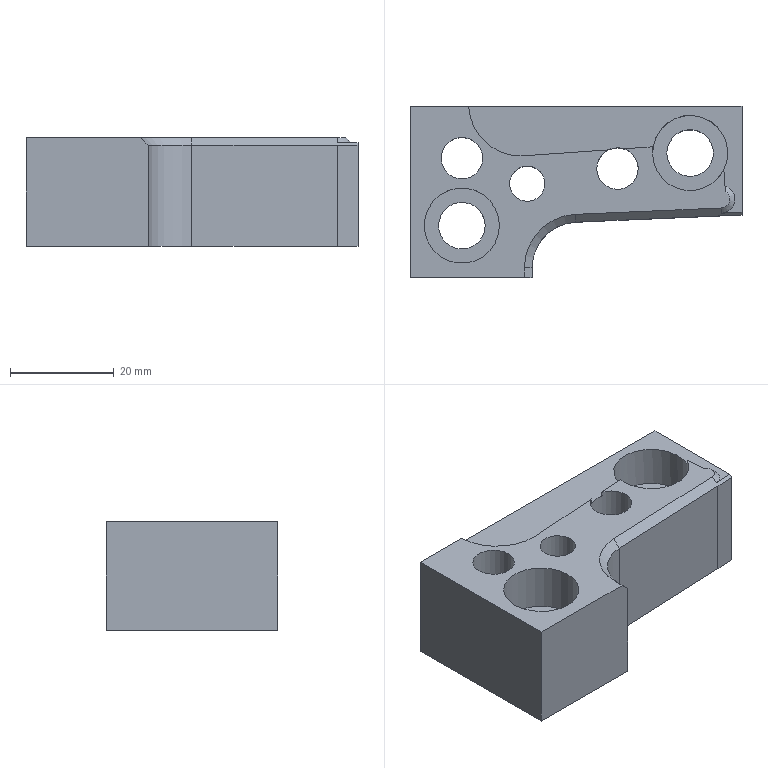Part | NX | features 23 2 | 1 solid | 28 faces | box 64 x 33 x 21 mm | volume 27332 mm3 | plane 17 | cylinder 9 | cone 2 | commonest cylinder face diameters 8.001 x2 9 x2 14.5 x2 6.8 x1 17.6 x1 19.999 x1
STEP:
#1=CARTESIAN_POINT('',(1071.25,364.,-2.5));
#2=VERTEX_POINT('',#1);
#3=CARTESIAN_POINT('',(1064.,364.,-2.5));
#4=DIRECTION('',(0.,0.,-1.));
#5=DIRECTION('',(1.,0.,0.));
#6=AXIS2_PLACEMENT_3D('',#3,#4,#5);
#7=CIRCLE('',#6,7.25);
#8=EDGE_CURVE('',#2,#2,#7,.T.);
#9=ORIENTED_EDGE('',*,*,#8,.T.);
#10=EDGE_LOOP('',(#9));
#11=FACE_BOUND('',#10,.T.);
#12=CARTESIAN_POINT('',(1068.001,377.,-2.5));
#13=VERTEX_POINT('',#12);
#14=CARTESIAN_POINT('',(1064.,377.,-2.5));
#15=DIRECTION('',(0.,0.,-1.));
#16=DIRECTION('',(1.,0.,0.));
#17=AXIS2_PLACEMENT_3D('',#14,#15,#16);
#18=CIRCLE('',#17,4.);
#19=EDGE_CURVE('',#13,#13,#18,.T.);
#20=ORIENTED_EDGE('',*,*,#19,.T.);
#21=EDGE_LOOP('',(#20));
#22=FACE_BOUND('',#21,.T.);
#23=CARTESIAN_POINT('',(1075.608,377.443,-2.5));
#24=VERTEX_POINT('',#23);
#25=CARTESIAN_POINT('',(1092.264,378.604,-2.5));
#26=VERTEX_POINT('',#25);
#27=CARTESIAN_POINT('',(1521.796,408.549,-2.5));
#28=DIRECTION('',(0.9976,0.06955,0.));
#29=VECTOR('',#28,1000.);
#30=LINE('',#27,#29);
#31=EDGE_CURVE('',#24,#26,#30,.T.);
#32=ORIENTED_EDGE('',*,*,#31,.F.);
#33=CARTESIAN_POINT('',(1065.29,387.,-2.5));
#34=VERTEX_POINT('',#33);
#35=CARTESIAN_POINT('',(1075.28,387.437,-2.5));
#36=DIRECTION('',(0.,0.,1.));
#37=DIRECTION('',(1.,0.,0.));
#38=AXIS2_PLACEMENT_3D('',#35,#36,#37);
#39=CIRCLE('',#38,10.);
#40=EDGE_CURVE('',#34,#24,#39,.T.);
#41=ORIENTED_EDGE('',*,*,#40,.F.);
#42=CARTESIAN_POINT('',(1054.,387.,-2.5));
#43=VERTEX_POINT('',#42);
#44=CARTESIAN_POINT('',(1136.,387.,-2.5));
#45=DIRECTION('',(-1.,0.,0.));
#46=VECTOR('',#45,1000.);
#47=LINE('',#44,#46);
#48=EDGE_CURVE('',#34,#43,#47,.T.);
#49=ORIENTED_EDGE('',*,*,#48,.T.);
#50=CARTESIAN_POINT('',(1054.,354.,-2.5));
#51=VERTEX_POINT('',#50);
#52=CARTESIAN_POINT('',(1054.,328.5,-2.5));
#53=DIRECTION('',(0.,-1.,0.));
#54=VECTOR('',#53,1000.);
#55=LINE('',#52,#54);
#56=EDGE_CURVE('',#43,#51,#55,.T.);
#57=ORIENTED_EDGE('',*,*,#56,.T.);
#58=CARTESIAN_POINT('',(1076.041,354.,-2.5));
#59=VERTEX_POINT('',#58);
#60=CARTESIAN_POINT('',(1166.5,354.,-2.5));
#61=DIRECTION('',(-1.,0.,0.));
#62=VECTOR('',#61,1000.);
#63=LINE('',#60,#62);
#64=EDGE_CURVE('',#59,#51,#63,.T.);
#65=ORIENTED_EDGE('',*,*,#64,.F.);
#66=CARTESIAN_POINT('',(1076.041,355.884,-2.5));
#67=VERTEX_POINT('',#66);
#68=CARTESIAN_POINT('',(1076.041,-425.,-2.5));
#69=DIRECTION('',(0.,1.,0.));
#70=VECTOR('',#69,1000.);
#71=LINE('',#68,#70);
#72=EDGE_CURVE('',#59,#67,#71,.T.);
#73=ORIENTED_EDGE('',*,*,#72,.T.);
#74=CARTESIAN_POINT('',(1085.893,366.175,-2.5));
#75=VERTEX_POINT('',#74);
#76=CARTESIAN_POINT('',(1086.341,355.884,-2.5));
#77=DIRECTION('',(0.,0.,1.));
#78=DIRECTION('',(1.,0.,0.));
#79=AXIS2_PLACEMENT_3D('',#76,#77,#78);
#80=CIRCLE('',#79,10.3);
#81=EDGE_CURVE('',#75,#67,#80,.T.);
#82=ORIENTED_EDGE('',*,*,#81,.F.);
#83=CARTESIAN_POINT('',(1113.99,367.4,-2.5));
#84=VERTEX_POINT('',#83);
#85=CARTESIAN_POINT('',(1544.537,386.173,-2.5));
#86=DIRECTION('',(0.9991,0.04356,0.));
#87=VECTOR('',#86,1000.);
#88=LINE('',#85,#87);
#89=EDGE_CURVE('',#75,#84,#88,.T.);
#90=ORIENTED_EDGE('',*,*,#89,.T.);
#91=CARTESIAN_POINT('',(1114.808,370.545,-2.5));
#92=VERTEX_POINT('',#91);
#93=CARTESIAN_POINT('',(1113.916,369.098,-2.5));
#94=DIRECTION('',(0.,0.,1.));
#95=DIRECTION('',(1.,0.,0.));
#96=AXIS2_PLACEMENT_3D('',#93,#94,#95);
#97=CIRCLE('',#96,1.7);
#98=EDGE_CURVE('',#84,#92,#97,.T.);
#99=ORIENTED_EDGE('',*,*,#98,.T.);
#100=CARTESIAN_POINT('',(1114.485,374.758,-2.5));
#101=VERTEX_POINT('',#100);
#102=CARTESIAN_POINT('',(1178.225,-455.826,-2.5));
#103=DIRECTION('',(0.07652,-0.9971,0.));
#104=VECTOR('',#103,1000.);
#105=LINE('',#102,#104);
#106=EDGE_CURVE('',#101,#92,#105,.T.);
#107=ORIENTED_EDGE('',*,*,#106,.F.);
#108=CARTESIAN_POINT('',(1100.85,379.203,-2.5));
#109=VERTEX_POINT('',#108);
#110=CARTESIAN_POINT('',(1108.,378.,-2.5));
#111=DIRECTION('',(0.,0.,-1.));
#112=DIRECTION('',(1.,0.,0.));
#113=AXIS2_PLACEMENT_3D('',#110,#111,#112);
#114=CIRCLE('',#113,7.25);
#115=EDGE_CURVE('',#101,#109,#114,.T.);
#116=ORIENTED_EDGE('',*,*,#115,.T.);
#117=CARTESIAN_POINT('',(1095.22,378.81,-2.5));
#118=VERTEX_POINT('',#117);
#119=CARTESIAN_POINT('',(1521.796,408.549,-2.5));
#120=DIRECTION('',(0.9976,0.06955,0.));
#121=VECTOR('',#120,1000.);
#122=LINE('',#119,#121);
#123=EDGE_CURVE('',#118,#109,#122,.T.);
#124=ORIENTED_EDGE('',*,*,#123,.F.);
#125=CARTESIAN_POINT('',(1094.,375.,-2.5));
#126=DIRECTION('',(0.,0.,-1.));
#127=DIRECTION('',(1.,0.,0.));
#128=AXIS2_PLACEMENT_3D('',#125,#126,#127);
#129=CIRCLE('',#128,4.);
#130=EDGE_CURVE('',#118,#26,#129,.T.);
#131=ORIENTED_EDGE('',*,*,#130,.T.);
#132=EDGE_LOOP('',(#32,#41,#49,#57,#65,#73,#82,#90,#99,#107,#116,#124,#131));
#133=FACE_BOUND('',#132,.T.);
#134=CARTESIAN_POINT('',(1079.999,372.088,-2.5));
#135=VERTEX_POINT('',#134);
#136=CARTESIAN_POINT('',(1076.599,372.088,-2.5));
#137=DIRECTION('',(0.,0.,1.));
#138=DIRECTION('',(1.,0.,0.));
#139=AXIS2_PLACEMENT_3D('',#136,#137,#138);
#140=CIRCLE('',#139,3.4);
#141=EDGE_CURVE('',#135,#135,#140,.T.);
#142=ORIENTED_EDGE('',*,*,#141,.F.);
#143=EDGE_LOOP('',(#142));
#144=FACE_BOUND('',#143,.T.);
#145=CARTESIAN_POINT('',(1166.5,279.5,-2.5));
#146=DIRECTION('',(0.,0.,1.));
#147=DIRECTION('',(-1.,0.,0.));
#148=AXIS2_PLACEMENT_3D('',#145,#146,#147);
#149=PLANE('',#148);
#150=ADVANCED_FACE('',(#11,#22,#133,#144),#149,.T.);
#151=ORIENTED_EDGE('',*,*,#123,.T.);
#152=CARTESIAN_POINT('',(1100.85,379.203,-3.5));
#153=VERTEX_POINT('',#152);
#154=CARTESIAN_POINT('',(1100.85,379.203,-3.5));
#155=DIRECTION('',(0.,0.,1.));
#156=VECTOR('',#155,1000.);
#157=LINE('',#154,#156);
#158=EDGE_CURVE('',#153,#109,#157,.T.);
#159=ORIENTED_EDGE('',*,*,#158,.F.);
#160=CARTESIAN_POINT('',(1095.22,378.81,-3.5));
#161=VERTEX_POINT('',#160);
#162=CARTESIAN_POINT('',(1580.768,412.66,-3.5));
#163=DIRECTION('',(0.9976,0.06955,0.));
#164=VECTOR('',#163,1000.);
#165=LINE('',#162,#164);
#166=EDGE_CURVE('',#161,#153,#165,.T.);
#167=ORIENTED_EDGE('',*,*,#166,.F.);
#168=CARTESIAN_POINT('',(1095.22,378.81,-0.5));
#169=DIRECTION('',(0.,0.,1.));
#170=VECTOR('',#169,1000.);
#171=LINE('',#168,#170);
#172=EDGE_CURVE('',#161,#118,#171,.T.);
#173=ORIENTED_EDGE('',*,*,#172,.T.);
#174=EDGE_LOOP('',(#151,#159,#167,#173));
#175=FACE_BOUND('',#174,.T.);
#176=CARTESIAN_POINT('',(1521.796,408.549,0.));
#177=DIRECTION('',(0.06955,-0.9976,0.));
#178=DIRECTION('',(0.9976,0.06955,0.));
#179=AXIS2_PLACEMENT_3D('',#176,#177,#178);
#180=PLANE('',#179);
#181=ADVANCED_FACE('',(#175),#180,.F.);
#182=CARTESIAN_POINT('',(1114.034,366.401,-3.5));
#183=VERTEX_POINT('',#182);
#184=CARTESIAN_POINT('',(1114.034,366.401,-3.5));
#185=DIRECTION('',(-0.0308,0.7064,0.7071));
#186=VECTOR('',#185,1000.);
#187=LINE('',#184,#186);
#188=EDGE_CURVE('',#183,#84,#187,.T.);
#189=ORIENTED_EDGE('',*,*,#188,.F.);
#190=CARTESIAN_POINT('',(1114.721,371.675,-3.5));
#191=VERTEX_POINT('',#190);
#192=CARTESIAN_POINT('',(1113.916,369.098,-3.5));
#193=DIRECTION('',(0.,0.,-1.));
#194=DIRECTION('',(-1.,0.,0.));
#195=AXIS2_PLACEMENT_3D('',#192,#193,#194);
#196=CIRCLE('',#195,2.7);
#197=EDGE_CURVE('',#191,#183,#196,.T.);
#198=ORIENTED_EDGE('',*,*,#197,.F.);
#199=CARTESIAN_POINT('',(1114.808,370.545,-2.5));
#200=CARTESIAN_POINT('',(1114.778,370.936,-2.817));
#201=CARTESIAN_POINT('',(1114.75,371.307,-3.157));
#202=CARTESIAN_POINT('',(1114.721,371.675,-3.5));
#203=B_SPLINE_CURVE_WITH_KNOTS('',3,(#199,#200,#201,#202),.UNSPECIFIED.,.F.,.F.,(4,4),(0.,0.001511),.UNSPECIFIED.);
#204=EDGE_CURVE('',#92,#191,#203,.T.);
#205=ORIENTED_EDGE('',*,*,#204,.F.);
#206=ORIENTED_EDGE('',*,*,#98,.F.);
#207=EDGE_LOOP('',(#189,#198,#205,#206));
#208=FACE_BOUND('',#207,.T.);
#209=CARTESIAN_POINT('',(1113.916,369.098,-3.5));
#210=DIRECTION('',(0.,0.,-1.));
#211=DIRECTION('',(-1.,0.,0.));
#212=AXIS2_PLACEMENT_3D('',#209,#210,#211);
#213=CONICAL_SURFACE('',#212,2.7,0.7854);
#214=ADVANCED_FACE('',(#208),#213,.T.);
#215=CARTESIAN_POINT('',(1065.29,387.,-3.5));
#216=VERTEX_POINT('',#215);
#217=CARTESIAN_POINT('',(1075.608,377.443,-3.5));
#218=VERTEX_POINT('',#217);
#219=CARTESIAN_POINT('',(1075.28,387.437,-3.5));
#220=DIRECTION('',(0.,0.,1.));
#221=DIRECTION('',(-1.,0.,0.));
#222=AXIS2_PLACEMENT_3D('',#219,#220,#221);
#223=CIRCLE('',#222,10.);
#224=EDGE_CURVE('',#216,#218,#223,.T.);
#225=ORIENTED_EDGE('',*,*,#224,.F.);
#226=CARTESIAN_POINT('',(1065.29,387.,0.));
#227=DIRECTION('',(0.,0.,-1.));
#228=VECTOR('',#227,1000.);
#229=LINE('',#226,#228);
#230=EDGE_CURVE('',#34,#216,#229,.T.);
#231=ORIENTED_EDGE('',*,*,#230,.F.);
#232=ORIENTED_EDGE('',*,*,#40,.T.);
#233=CARTESIAN_POINT('',(1075.608,377.443,-3.5));
#234=DIRECTION('',(0.,0.,-1.));
#235=VECTOR('',#234,1000.);
#236=LINE('',#233,#235);
#237=EDGE_CURVE('',#24,#218,#236,.T.);
#238=ORIENTED_EDGE('',*,*,#237,.T.);
#239=EDGE_LOOP('',(#225,#231,#232,#238));
#240=FACE_BOUND('',#239,.T.);
#241=CARTESIAN_POINT('',(1075.28,387.437,0.));
#242=DIRECTION('',(0.,0.,-1.));
#243=DIRECTION('',(-1.,0.,0.));
#244=AXIS2_PLACEMENT_3D('',#241,#242,#243);
#245=CYLINDRICAL_SURFACE('',#244,10.);
#246=ADVANCED_FACE('',(#240),#245,.F.);
#247=CARTESIAN_POINT('',(1092.264,378.604,-3.5));
#248=VERTEX_POINT('',#247);
#249=CARTESIAN_POINT('',(1092.264,378.604,-0.5));
#250=DIRECTION('',(0.,0.,-1.));
#251=VECTOR('',#250,1000.);
#252=LINE('',#249,#251);
#253=EDGE_CURVE('',#26,#248,#252,.T.);
#254=ORIENTED_EDGE('',*,*,#253,.T.);
#255=CARTESIAN_POINT('',(1580.768,412.66,-3.5));
#256=DIRECTION('',(0.9976,0.06955,0.));
#257=VECTOR('',#256,1000.);
#258=LINE('',#255,#257);
#259=EDGE_CURVE('',#218,#248,#258,.T.);
#260=ORIENTED_EDGE('',*,*,#259,.F.);
#261=ORIENTED_EDGE('',*,*,#237,.F.);
#262=ORIENTED_EDGE('',*,*,#31,.T.);
#263=EDGE_LOOP('',(#254,#260,#261,#262));
#264=FACE_BOUND('',#263,.T.);
#265=CARTESIAN_POINT('',(1521.796,408.549,0.));
#266=DIRECTION('',(0.06955,-0.9976,0.));
#267=DIRECTION('',(0.9976,0.06955,0.));
#268=AXIS2_PLACEMENT_3D('',#265,#266,#267);
#269=PLANE('',#268);
#270=ADVANCED_FACE('',(#264),#269,.F.);
#271=ORIENTED_EDGE('',*,*,#106,.T.);
#272=ORIENTED_EDGE('',*,*,#204,.T.);
#273=CARTESIAN_POINT('',(1114.485,374.758,-3.5));
#274=VERTEX_POINT('',#273);
#275=CARTESIAN_POINT('',(1113.377,389.198,-3.5));
#276=DIRECTION('',(0.07652,-0.9971,0.));
#277=VECTOR('',#276,1000.);
#278=LINE('',#275,#277);
#279=EDGE_CURVE('',#274,#191,#278,.T.);
#280=ORIENTED_EDGE('',*,*,#279,.F.);
#281=CARTESIAN_POINT('',(1114.485,374.758,-2.5));
#282=DIRECTION('',(0.,0.,-1.));
#283=VECTOR('',#282,1000.);
#284=LINE('',#281,#283);
#285=EDGE_CURVE('',#101,#274,#284,.T.);
#286=ORIENTED_EDGE('',*,*,#285,.F.);
#287=EDGE_LOOP('',(#271,#272,#280,#286));
#288=FACE_BOUND('',#287,.T.);
#289=CARTESIAN_POINT('',(1178.225,-455.826,0.));
#290=DIRECTION('',(-0.9971,-0.07652,0.));
#291=DIRECTION('',(0.07652,-0.9971,0.));
#292=AXIS2_PLACEMENT_3D('',#289,#290,#291);
#293=PLANE('',#292);
#294=ADVANCED_FACE('',(#288),#293,.F.);
#295=CARTESIAN_POINT('',(1118.,387.,-3.5));
#296=VERTEX_POINT('',#295);
#297=CARTESIAN_POINT('',(1118.,366.574,-3.5));
#298=VERTEX_POINT('',#297);
#299=CARTESIAN_POINT('',(1118.,332.,-3.5));
#300=DIRECTION('',(0.,-1.,0.));
#301=VECTOR('',#300,1000.);
#302=LINE('',#299,#301);
#303=EDGE_CURVE('',#296,#298,#302,.T.);
#304=ORIENTED_EDGE('',*,*,#303,.T.);
#305=CARTESIAN_POINT('',(1118.,366.073,-4.));
#306=VERTEX_POINT('',#305);
#307=CARTESIAN_POINT('',(1118.,351.02,-19.038));
#308=DIRECTION('',(0.,0.7074,0.7068));
#309=VECTOR('',#308,1000.);
#310=LINE('',#307,#309);
#311=EDGE_CURVE('',#306,#298,#310,.T.);
#312=ORIENTED_EDGE('',*,*,#311,.F.);
#313=CARTESIAN_POINT('',(1118.,366.073,-23.5));
#314=VERTEX_POINT('',#313);
#315=CARTESIAN_POINT('',(1118.,366.073,0.));
#316=DIRECTION('',(0.,0.,-1.));
#317=VECTOR('',#316,1000.);
#318=LINE('',#315,#317);
#319=EDGE_CURVE('',#306,#314,#318,.T.);
#320=ORIENTED_EDGE('',*,*,#319,.T.);
#321=CARTESIAN_POINT('',(1118.,387.,-23.5));
#322=VERTEX_POINT('',#321);
#323=CARTESIAN_POINT('',(1118.,328.5,-23.5));
#324=DIRECTION('',(0.,-1.,0.));
#325=VECTOR('',#324,1000.);
#326=LINE('',#323,#325);
#327=EDGE_CURVE('',#322,#314,#326,.T.);
#328=ORIENTED_EDGE('',*,*,#327,.F.);
#329=CARTESIAN_POINT('',(1118.,387.,-33.5));
#330=DIRECTION('',(0.,0.,1.));
#331=VECTOR('',#330,1000.);
#332=LINE('',#329,#331);
#333=EDGE_CURVE('',#322,#296,#332,.T.);
#334=ORIENTED_EDGE('',*,*,#333,.T.);
#335=EDGE_LOOP('',(#304,#312,#320,#328,#334));
#336=FACE_BOUND('',#335,.T.);
#337=CARTESIAN_POINT('',(1118.,332.,0.));
#338=DIRECTION('',(1.,0.,0.));
#339=DIRECTION('',(0.,0.,1.));
#340=AXIS2_PLACEMENT_3D('',#337,#338,#339);
#341=PLANE('',#340);
#342=ADVANCED_FACE('',(#336),#341,.T.);
#343=CARTESIAN_POINT('',(1073.199,372.088,-23.5));
#344=VERTEX_POINT('',#343);
#345=CARTESIAN_POINT('',(1076.599,372.088,-23.5));
#346=DIRECTION('',(0.,0.,1.));
#347=DIRECTION('',(-1.,0.,0.));
#348=AXIS2_PLACEMENT_3D('',#345,#346,#347);
#349=CIRCLE('',#348,3.4);
#350=EDGE_CURVE('',#344,#344,#349,.T.);
#351=ORIENTED_EDGE('',*,*,#350,.T.);
#352=EDGE_LOOP('',(#351));
#353=FACE_BOUND('',#352,.T.);
#354=CARTESIAN_POINT('',(1090.,375.,-23.5));
#355=VERTEX_POINT('',#354);
#356=CARTESIAN_POINT('',(1094.,375.,-23.5));
#357=DIRECTION('',(0.,0.,1.));
#358=DIRECTION('',(-1.,0.,0.));
#359=AXIS2_PLACEMENT_3D('',#356,#357,#358);
#360=CIRCLE('',#359,4.);
#361=EDGE_CURVE('',#355,#355,#360,.T.);
#362=ORIENTED_EDGE('',*,*,#361,.T.);
#363=EDGE_LOOP('',(#362));
#364=FACE_BOUND('',#363,.T.);
#365=CARTESIAN_POINT('',(1059.999,377.,-23.5));
#366=VERTEX_POINT('',#365);
#367=CARTESIAN_POINT('',(1064.,377.,-23.5));
#368=DIRECTION('',(0.,0.,1.));
#369=DIRECTION('',(-1.,0.,0.));
#370=AXIS2_PLACEMENT_3D('',#367,#368,#369);
#371=CIRCLE('',#370,4.);
#372=EDGE_CURVE('',#366,#366,#371,.T.);
#373=ORIENTED_EDGE('',*,*,#372,.T.);
#374=EDGE_LOOP('',(#373));
#375=FACE_BOUND('',#374,.T.);
#376=CARTESIAN_POINT('',(1059.5,364.,-23.5));
#377=VERTEX_POINT('',#376);
#378=CARTESIAN_POINT('',(1064.,364.,-23.5));
#379=DIRECTION('',(0.,0.,1.));
#380=DIRECTION('',(-1.,0.,0.));
#381=AXIS2_PLACEMENT_3D('',#378,#379,#380);
#382=CIRCLE('',#381,4.5);
#383=EDGE_CURVE('',#377,#377,#382,.T.);
#384=ORIENTED_EDGE('',*,*,#383,.T.);
#385=EDGE_LOOP('',(#384));
#386=FACE_BOUND('',#385,.T.);
#387=CARTESIAN_POINT('',(1103.5,378.,-23.5));
#388=VERTEX_POINT('',#387);
#389=CARTESIAN_POINT('',(1108.,378.,-23.5));
#390=DIRECTION('',(0.,0.,1.));
#391=DIRECTION('',(-1.,0.,0.));
#392=AXIS2_PLACEMENT_3D('',#389,#390,#391);
#393=CIRCLE('',#392,4.5);
#394=EDGE_CURVE('',#388,#388,#393,.T.);
#395=ORIENTED_EDGE('',*,*,#394,.T.);
#396=EDGE_LOOP('',(#395));
#397=FACE_BOUND('',#396,.T.);
#398=CARTESIAN_POINT('',(1054.,354.,-23.5));
#399=VERTEX_POINT('',#398);
#400=CARTESIAN_POINT('',(1077.541,354.,-23.5));
#401=VERTEX_POINT('',#400);
#402=CARTESIAN_POINT('',(1136.,354.,-23.5));
#403=DIRECTION('',(1.,0.,0.));
#404=VECTOR('',#403,1000.);
#405=LINE('',#402,#404);
#406=EDGE_CURVE('',#399,#401,#405,.T.);
#407=ORIENTED_EDGE('',*,*,#406,.F.);
#408=CARTESIAN_POINT('',(1054.,387.,-23.5));
#409=VERTEX_POINT('',#408);
#410=CARTESIAN_POINT('',(1054.,328.5,-23.5));
#411=DIRECTION('',(0.,1.,0.));
#412=VECTOR('',#411,1000.);
#413=LINE('',#410,#412);
#414=EDGE_CURVE('',#399,#409,#413,.T.);
#415=ORIENTED_EDGE('',*,*,#414,.T.);
#416=CARTESIAN_POINT('',(1136.,387.,-23.5));
#417=DIRECTION('',(1.,0.,0.));
#418=VECTOR('',#417,1000.);
#419=LINE('',#416,#418);
#420=EDGE_CURVE('',#409,#322,#419,.T.);
#421=ORIENTED_EDGE('',*,*,#420,.T.);
#422=ORIENTED_EDGE('',*,*,#327,.T.);
#423=CARTESIAN_POINT('',(1114.056,365.901,-23.5));
#424=VERTEX_POINT('',#423);
#425=CARTESIAN_POINT('',(1134.331,366.785,-23.5));
#426=DIRECTION('',(0.9991,0.04356,0.));
#427=VECTOR('',#426,1000.);
#428=LINE('',#425,#427);
#429=EDGE_CURVE('',#424,#314,#428,.T.);
#430=ORIENTED_EDGE('',*,*,#429,.F.);
#431=CARTESIAN_POINT('',(1085.958,364.676,-23.5));
#432=VERTEX_POINT('',#431);
#433=CARTESIAN_POINT('',(1134.331,366.785,-23.5));
#434=DIRECTION('',(0.9991,0.04356,0.));
#435=VECTOR('',#434,1000.);
#436=LINE('',#433,#435);
#437=EDGE_CURVE('',#432,#424,#436,.T.);
#438=ORIENTED_EDGE('',*,*,#437,.F.);
#439=CARTESIAN_POINT('',(1077.541,355.884,-23.5));
#440=VERTEX_POINT('',#439);
#441=CARTESIAN_POINT('',(1086.341,355.884,-23.5));
#442=DIRECTION('',(0.,0.,1.));
#443=DIRECTION('',(-1.,0.,0.));
#444=AXIS2_PLACEMENT_3D('',#441,#442,#443);
#445=CIRCLE('',#444,8.8);
#446=EDGE_CURVE('',#432,#440,#445,.T.);
#447=ORIENTED_EDGE('',*,*,#446,.T.);
#448=CARTESIAN_POINT('',(1077.541,328.5,-23.5));
#449=DIRECTION('',(0.,-1.,0.));
#450=VECTOR('',#449,1000.);
#451=LINE('',#448,#450);
#452=EDGE_CURVE('',#440,#401,#451,.T.);
#453=ORIENTED_EDGE('',*,*,#452,.T.);
#454=EDGE_LOOP('',(#407,#415,#421,#422,#430,#438,#447,#453));
#455=FACE_BOUND('',#454,.T.);
#456=CARTESIAN_POINT('',(1136.,328.5,-23.5));
#457=DIRECTION('',(0.,0.,-1.));
#458=DIRECTION('',(1.,0.,0.));
#459=AXIS2_PLACEMENT_3D('',#456,#457,#458);
#460=PLANE('',#459);
#461=ADVANCED_FACE('',(#353,#364,#375,#386,#397,#455),#460,.T.);
#462=CARTESIAN_POINT('',(1054.,387.,-33.5));
#463=DIRECTION('',(0.,0.,-1.));
#464=VECTOR('',#463,1000.);
#465=LINE('',#462,#464);
#466=EDGE_CURVE('',#43,#409,#465,.T.);
#467=ORIENTED_EDGE('',*,*,#466,.F.);
#468=ORIENTED_EDGE('',*,*,#48,.F.);
#469=ORIENTED_EDGE('',*,*,#230,.T.);
#470=CARTESIAN_POINT('',(1136.,387.,-3.5));
#471=DIRECTION('',(1.,0.,0.));
#472=VECTOR('',#471,1000.);
#473=LINE('',#470,#472);
#474=EDGE_CURVE('',#216,#296,#473,.T.);
#475=ORIENTED_EDGE('',*,*,#474,.T.);
#476=ORIENTED_EDGE('',*,*,#333,.F.);
#477=ORIENTED_EDGE('',*,*,#420,.F.);
#478=EDGE_LOOP('',(#467,#468,#469,#475,#476,#477));
#479=FACE_BOUND('',#478,.T.);
#480=CARTESIAN_POINT('',(1136.,387.,-33.5));
#481=DIRECTION('',(0.,1.,0.));
#482=DIRECTION('',(0.,0.,-1.));
#483=AXIS2_PLACEMENT_3D('',#480,#481,#482);
#484=PLANE('',#483);
#485=ADVANCED_FACE('',(#479),#484,.T.);
#486=CARTESIAN_POINT('',(1054.,354.,-33.5));
#487=DIRECTION('',(0.,0.,1.));
#488=VECTOR('',#487,1000.);
#489=LINE('',#486,#488);
#490=EDGE_CURVE('',#399,#51,#489,.T.);
#491=ORIENTED_EDGE('',*,*,#490,.T.);
#492=ORIENTED_EDGE('',*,*,#56,.F.);
#493=ORIENTED_EDGE('',*,*,#466,.T.);
#494=ORIENTED_EDGE('',*,*,#414,.F.);
#495=EDGE_LOOP('',(#491,#492,#493,#494));
#496=FACE_BOUND('',#495,.T.);
#497=CARTESIAN_POINT('',(1054.,328.5,-33.5));
#498=DIRECTION('',(-1.,0.,0.));
#499=DIRECTION('',(0.,0.,-1.));
#500=AXIS2_PLACEMENT_3D('',#497,#498,#499);
#501=PLANE('',#500);
#502=ADVANCED_FACE('',(#496),#501,.T.);
#503=CARTESIAN_POINT('',(1077.541,354.,-4.));
#504=VERTEX_POINT('',#503);
#505=CARTESIAN_POINT('',(1077.041,354.,-3.5));
#506=DIRECTION('',(-0.7071,0.,0.7071));
#507=VECTOR('',#506,1000.);
#508=LINE('',#505,#507);
#509=EDGE_CURVE('',#504,#59,#508,.T.);
#510=ORIENTED_EDGE('',*,*,#509,.F.);
#511=CARTESIAN_POINT('',(1077.541,355.884,-4.));
#512=VERTEX_POINT('',#511);
#513=CARTESIAN_POINT('',(1077.541,-425.,-4.));
#514=DIRECTION('',(0.,-1.,0.));
#515=VECTOR('',#514,1000.);
#516=LINE('',#513,#515);
#517=EDGE_CURVE('',#512,#504,#516,.T.);
#518=ORIENTED_EDGE('',*,*,#517,.F.);
#519=CARTESIAN_POINT('',(1077.041,355.884,-3.5));
#520=DIRECTION('',(-0.7071,0.,0.7071));
#521=VECTOR('',#520,1000.);
#522=LINE('',#519,#521);
#523=EDGE_CURVE('',#512,#67,#522,.T.);
#524=ORIENTED_EDGE('',*,*,#523,.T.);
#525=ORIENTED_EDGE('',*,*,#72,.F.);
#526=EDGE_LOOP('',(#510,#518,#524,#525));
#527=FACE_BOUND('',#526,.T.);
#528=CARTESIAN_POINT('',(1077.041,-425.,-3.5));
#529=DIRECTION('',(0.7071,0.,0.7071));
#530=DIRECTION('',(0.,-1.,0.));
#531=AXIS2_PLACEMENT_3D('',#528,#529,#530);
#532=PLANE('',#531);
#533=ADVANCED_FACE('',(#527),#532,.T.);
#534=ORIENTED_EDGE('',*,*,#81,.T.);
#535=ORIENTED_EDGE('',*,*,#523,.F.);
#536=CARTESIAN_POINT('',(1085.958,364.676,-4.));
#537=VERTEX_POINT('',#536);
#538=CARTESIAN_POINT('',(1086.341,355.884,-4.));
#539=DIRECTION('',(0.,0.,1.));
#540=DIRECTION('',(-1.,0.,0.));
#541=AXIS2_PLACEMENT_3D('',#538,#539,#540);
#542=CIRCLE('',#541,8.8);
#543=EDGE_CURVE('',#537,#512,#542,.T.);
#544=ORIENTED_EDGE('',*,*,#543,.F.);
#545=CARTESIAN_POINT('',(1085.936,365.176,-3.5));
#546=DIRECTION('',(-0.0308,0.7064,0.7071));
#547=VECTOR('',#546,1000.);
#548=LINE('',#545,#547);
#549=EDGE_CURVE('',#537,#75,#548,.T.);
#550=ORIENTED_EDGE('',*,*,#549,.T.);
#551=EDGE_LOOP('',(#534,#535,#544,#550));
#552=FACE_BOUND('',#551,.T.);
#553=CARTESIAN_POINT('',(1086.341,355.884,-3.5));
#554=DIRECTION('',(0.,0.,1.));
#555=DIRECTION('',(1.,0.,0.));
#556=AXIS2_PLACEMENT_3D('',#553,#554,#555);
#557=CONICAL_SURFACE('',#556,9.3,0.7854);
#558=ADVANCED_FACE('',(#552),#557,.F.);
#559=ORIENTED_EDGE('',*,*,#188,.T.);
#560=ORIENTED_EDGE('',*,*,#89,.F.);
#561=ORIENTED_EDGE('',*,*,#549,.F.);
#562=CARTESIAN_POINT('',(1114.056,365.901,-4.));
#563=VERTEX_POINT('',#562);
#564=CARTESIAN_POINT('',(1544.602,384.675,-4.));
#565=DIRECTION('',(-0.9991,-0.04356,0.));
#566=VECTOR('',#565,1000.);
#567=LINE('',#564,#566);
#568=EDGE_CURVE('',#563,#537,#567,.T.);
#569=ORIENTED_EDGE('',*,*,#568,.F.);
#570=CARTESIAN_POINT('',(1114.056,365.901,-4.));
#571=DIRECTION('',(0.9991,0.04356,0.));
#572=VECTOR('',#571,1000.);
#573=LINE('',#570,#572);
#574=EDGE_CURVE('',#563,#306,#573,.T.);
#575=ORIENTED_EDGE('',*,*,#574,.T.);
#576=ORIENTED_EDGE('',*,*,#311,.T.);
#577=CARTESIAN_POINT('',(1544.581,385.174,-3.5));
#578=DIRECTION('',(-0.9991,-0.04356,0.));
#579=VECTOR('',#578,1000.);
#580=LINE('',#577,#579);
#581=EDGE_CURVE('',#298,#183,#580,.T.);
#582=ORIENTED_EDGE('',*,*,#581,.T.);
#583=EDGE_LOOP('',(#559,#560,#561,#569,#575,#576,#582));
#584=FACE_BOUND('',#583,.T.);
#585=CARTESIAN_POINT('',(1544.581,385.174,-3.5));
#586=DIRECTION('',(0.0308,-0.7064,0.7071));
#587=DIRECTION('',(-0.9991,-0.04356,0.));
#588=AXIS2_PLACEMENT_3D('',#585,#586,#587);
#589=PLANE('',#588);
#590=ADVANCED_FACE('',(#584),#589,.T.);
#591=CARTESIAN_POINT('',(1077.541,354.,-43.));
#592=DIRECTION('',(0.,0.,-1.));
#593=VECTOR('',#592,1000.);
#594=LINE('',#591,#593);
#595=EDGE_CURVE('',#504,#401,#594,.T.);
#596=ORIENTED_EDGE('',*,*,#595,.T.);
#597=ORIENTED_EDGE('',*,*,#452,.F.);
#598=CARTESIAN_POINT('',(1077.541,355.884,-43.));
#599=DIRECTION('',(0.,0.,-1.));
#600=VECTOR('',#599,1000.);
#601=LINE('',#598,#600);
#602=EDGE_CURVE('',#512,#440,#601,.T.);
#603=ORIENTED_EDGE('',*,*,#602,.F.);
#604=ORIENTED_EDGE('',*,*,#517,.T.);
#605=EDGE_LOOP('',(#596,#597,#603,#604));
#606=FACE_BOUND('',#605,.T.);
#607=CARTESIAN_POINT('',(1077.541,275.983,-43.));
#608=DIRECTION('',(1.,0.,0.));
#609=DIRECTION('',(0.,0.,1.));
#610=AXIS2_PLACEMENT_3D('',#607,#608,#609);
#611=PLANE('',#610);
#612=ADVANCED_FACE('',(#606),#611,.T.);
#613=ORIENTED_EDGE('',*,*,#446,.F.);
#614=CARTESIAN_POINT('',(1085.958,364.676,-43.));
#615=DIRECTION('',(0.,0.,-1.));
#616=VECTOR('',#615,1000.);
#617=LINE('',#614,#616);
#618=EDGE_CURVE('',#537,#432,#617,.T.);
#619=ORIENTED_EDGE('',*,*,#618,.F.);
#620=ORIENTED_EDGE('',*,*,#543,.T.);
#621=ORIENTED_EDGE('',*,*,#602,.T.);
#622=EDGE_LOOP('',(#613,#619,#620,#621));
#623=FACE_BOUND('',#622,.T.);
#624=CARTESIAN_POINT('',(1086.341,355.884,-43.));
#625=DIRECTION('',(0.,0.,1.));
#626=DIRECTION('',(-1.,0.,0.));
#627=AXIS2_PLACEMENT_3D('',#624,#625,#626);
#628=CYLINDRICAL_SURFACE('',#627,8.8);
#629=ADVANCED_FACE('',(#623),#628,.F.);
#630=ORIENTED_EDGE('',*,*,#437,.T.);
#631=CARTESIAN_POINT('',(1114.056,365.901,-43.));
#632=DIRECTION('',(0.,0.,-1.));
#633=VECTOR('',#632,1000.);
#634=LINE('',#631,#633);
#635=EDGE_CURVE('',#563,#424,#634,.T.);
#636=ORIENTED_EDGE('',*,*,#635,.F.);
#637=ORIENTED_EDGE('',*,*,#568,.T.);
#638=ORIENTED_EDGE('',*,*,#618,.T.);
#639=EDGE_LOOP('',(#630,#636,#637,#638));
#640=FACE_BOUND('',#639,.T.);
#641=CARTESIAN_POINT('',(1085.958,364.676,-43.));
#642=DIRECTION('',(0.04356,-0.9991,0.));
#643=DIRECTION('',(-0.9991,-0.04356,0.));
#644=AXIS2_PLACEMENT_3D('',#641,#642,#643);
#645=PLANE('',#644);
#646=ADVANCED_FACE('',(#640),#645,.T.);
#647=ORIENTED_EDGE('',*,*,#319,.F.);
#648=ORIENTED_EDGE('',*,*,#574,.F.);
#649=ORIENTED_EDGE('',*,*,#635,.T.);
#650=ORIENTED_EDGE('',*,*,#429,.T.);
#651=EDGE_LOOP('',(#647,#648,#649,#650));
#652=FACE_BOUND('',#651,.T.);
#653=CARTESIAN_POINT('',(1114.056,365.901,-43.));
#654=DIRECTION('',(0.04356,-0.9991,0.));
#655=DIRECTION('',(-0.9991,-0.04356,0.));
#656=AXIS2_PLACEMENT_3D('',#653,#654,#655);
#657=PLANE('',#656);
#658=ADVANCED_FACE('',(#652),#657,.T.);
#659=CARTESIAN_POINT('',(1094.,375.,-3.5));
#660=DIRECTION('',(0.,0.,-1.));
#661=DIRECTION('',(-1.,0.,0.));
#662=AXIS2_PLACEMENT_3D('',#659,#660,#661);
#663=CIRCLE('',#662,4.);
#664=EDGE_CURVE('',#248,#161,#663,.T.);
#665=ORIENTED_EDGE('',*,*,#664,.T.);
#666=ORIENTED_EDGE('',*,*,#166,.T.);
#667=CARTESIAN_POINT('',(1108.,378.,-3.5));
#668=DIRECTION('',(0.,0.,1.));
#669=DIRECTION('',(-1.,0.,0.));
#670=AXIS2_PLACEMENT_3D('',#667,#668,#669);
#671=CIRCLE('',#670,7.25);
#672=EDGE_CURVE('',#274,#153,#671,.T.);
#673=ORIENTED_EDGE('',*,*,#672,.F.);
#674=ORIENTED_EDGE('',*,*,#279,.T.);
#675=ORIENTED_EDGE('',*,*,#197,.T.);
#676=ORIENTED_EDGE('',*,*,#581,.F.);
#677=ORIENTED_EDGE('',*,*,#303,.F.);
#678=ORIENTED_EDGE('',*,*,#474,.F.);
#679=ORIENTED_EDGE('',*,*,#224,.T.);
#680=ORIENTED_EDGE('',*,*,#259,.T.);
#681=EDGE_LOOP('',(#665,#666,#673,#674,#675,#676,#677,#678,#679,#680));
#682=FACE_BOUND('',#681,.T.);
#683=CARTESIAN_POINT('',(1579.908,425.,-3.5));
#684=DIRECTION('',(0.,0.,-1.));
#685=DIRECTION('',(1.,0.,0.));
#686=AXIS2_PLACEMENT_3D('',#683,#684,#685);
#687=PLANE('',#686);
#688=ADVANCED_FACE('',(#682),#687,.F.);
#689=ORIENTED_EDGE('',*,*,#490,.F.);
#690=ORIENTED_EDGE('',*,*,#406,.T.);
#691=ORIENTED_EDGE('',*,*,#595,.F.);
#692=ORIENTED_EDGE('',*,*,#509,.T.);
#693=ORIENTED_EDGE('',*,*,#64,.T.);
#694=EDGE_LOOP('',(#689,#690,#691,#692,#693));
#695=FACE_BOUND('',#694,.T.);
#696=CARTESIAN_POINT('',(1033.,354.,0.));
#697=DIRECTION('',(0.,1.,0.));
#698=DIRECTION('',(0.,0.,-1.));
#699=AXIS2_PLACEMENT_3D('',#696,#697,#698);
#700=PLANE('',#699);
#701=ADVANCED_FACE('',(#695),#700,.F.);
#702=ORIENTED_EDGE('',*,*,#394,.F.);
#703=EDGE_LOOP('',(#702));
#704=FACE_BOUND('',#703,.T.);
#705=CARTESIAN_POINT('',(1103.5,378.,-11.5));
#706=VERTEX_POINT('',#705);
#707=CARTESIAN_POINT('',(1108.,378.,-11.5));
#708=DIRECTION('',(0.,0.,1.));
#709=DIRECTION('',(-1.,0.,0.));
#710=AXIS2_PLACEMENT_3D('',#707,#708,#709);
#711=CIRCLE('',#710,4.5);
#712=EDGE_CURVE('',#706,#706,#711,.T.);
#713=ORIENTED_EDGE('',*,*,#712,.T.);
#714=EDGE_LOOP('',(#713));
#715=FACE_BOUND('',#714,.T.);
#716=CARTESIAN_POINT('',(1108.,378.,-0.5));
#717=DIRECTION('',(0.,0.,-1.));
#718=DIRECTION('',(-1.,0.,0.));
#719=AXIS2_PLACEMENT_3D('',#716,#717,#718);
#720=CYLINDRICAL_SURFACE('',#719,4.5);
#721=ADVANCED_FACE('',(#704,#715),#720,.F.);
#722=ORIENTED_EDGE('',*,*,#712,.F.);
#723=EDGE_LOOP('',(#722));
#724=FACE_BOUND('',#723,.T.);
#725=CARTESIAN_POINT('',(1100.75,378.,-11.5));
#726=VERTEX_POINT('',#725);
#727=CARTESIAN_POINT('',(1108.,378.,-11.5));
#728=DIRECTION('',(0.,0.,1.));
#729=DIRECTION('',(-1.,0.,0.));
#730=AXIS2_PLACEMENT_3D('',#727,#728,#729);
#731=CIRCLE('',#730,7.25);
#732=EDGE_CURVE('',#726,#726,#731,.T.);
#733=ORIENTED_EDGE('',*,*,#732,.T.);
#734=EDGE_LOOP('',(#733));
#735=FACE_BOUND('',#734,.T.);
#736=CARTESIAN_POINT('',(1108.,378.,-11.5));
#737=DIRECTION('',(0.,0.,-1.));
#738=DIRECTION('',(1.,0.,0.));
#739=AXIS2_PLACEMENT_3D('',#736,#737,#738);
#740=PLANE('',#739);
#741=ADVANCED_FACE('',(#724,#735),#740,.F.);
#742=ORIENTED_EDGE('',*,*,#672,.T.);
#743=ORIENTED_EDGE('',*,*,#158,.T.);
#744=ORIENTED_EDGE('',*,*,#115,.F.);
#745=ORIENTED_EDGE('',*,*,#285,.T.);
#746=EDGE_LOOP('',(#742,#743,#744,#745));
#747=FACE_BOUND('',#746,.T.);
#748=ORIENTED_EDGE('',*,*,#732,.F.);
#749=EDGE_LOOP('',(#748));
#750=FACE_BOUND('',#749,.T.);
#751=CARTESIAN_POINT('',(1108.,378.,-2.5));
#752=DIRECTION('',(0.,0.,-1.));
#753=DIRECTION('',(-1.,0.,0.));
#754=AXIS2_PLACEMENT_3D('',#751,#752,#753);
#755=CYLINDRICAL_SURFACE('',#754,7.25);
#756=ADVANCED_FACE('',(#747,#750),#755,.F.);
#757=ORIENTED_EDGE('',*,*,#383,.F.);
#758=EDGE_LOOP('',(#757));
#759=FACE_BOUND('',#758,.T.);
#760=CARTESIAN_POINT('',(1059.5,364.,-11.5));
#761=VERTEX_POINT('',#760);
#762=CARTESIAN_POINT('',(1064.,364.,-11.5));
#763=DIRECTION('',(0.,0.,1.));
#764=DIRECTION('',(-1.,0.,0.));
#765=AXIS2_PLACEMENT_3D('',#762,#763,#764);
#766=CIRCLE('',#765,4.5);
#767=EDGE_CURVE('',#761,#761,#766,.T.);
#768=ORIENTED_EDGE('',*,*,#767,.T.);
#769=EDGE_LOOP('',(#768));
#770=FACE_BOUND('',#769,.T.);
#771=CARTESIAN_POINT('',(1064.,364.,-0.5));
#772=DIRECTION('',(0.,0.,-1.));
#773=DIRECTION('',(-1.,0.,0.));
#774=AXIS2_PLACEMENT_3D('',#771,#772,#773);
#775=CYLINDRICAL_SURFACE('',#774,4.5);
#776=ADVANCED_FACE('',(#759,#770),#775,.F.);
#777=ORIENTED_EDGE('',*,*,#767,.F.);
#778=EDGE_LOOP('',(#777));
#779=FACE_BOUND('',#778,.T.);
#780=CARTESIAN_POINT('',(1056.75,364.,-11.5));
#781=VERTEX_POINT('',#780);
#782=CARTESIAN_POINT('',(1064.,364.,-11.5));
#783=DIRECTION('',(0.,0.,1.));
#784=DIRECTION('',(-1.,0.,0.));
#785=AXIS2_PLACEMENT_3D('',#782,#783,#784);
#786=CIRCLE('',#785,7.25);
#787=EDGE_CURVE('',#781,#781,#786,.T.);
#788=ORIENTED_EDGE('',*,*,#787,.T.);
#789=EDGE_LOOP('',(#788));
#790=FACE_BOUND('',#789,.T.);
#791=CARTESIAN_POINT('',(1064.,364.,-11.5));
#792=DIRECTION('',(0.,0.,-1.));
#793=DIRECTION('',(1.,0.,0.));
#794=AXIS2_PLACEMENT_3D('',#791,#792,#793);
#795=PLANE('',#794);
#796=ADVANCED_FACE('',(#779,#790),#795,.F.);
#797=ORIENTED_EDGE('',*,*,#8,.F.);
#798=EDGE_LOOP('',(#797));
#799=FACE_BOUND('',#798,.T.);
#800=ORIENTED_EDGE('',*,*,#787,.F.);
#801=EDGE_LOOP('',(#800));
#802=FACE_BOUND('',#801,.T.);
#803=CARTESIAN_POINT('',(1064.,364.,-2.5));
#804=DIRECTION('',(0.,0.,-1.));
#805=DIRECTION('',(-1.,0.,0.));
#806=AXIS2_PLACEMENT_3D('',#803,#804,#805);
#807=CYLINDRICAL_SURFACE('',#806,7.25);
#808=ADVANCED_FACE('',(#799,#802),#807,.F.);
#809=ORIENTED_EDGE('',*,*,#372,.F.);
#810=EDGE_LOOP('',(#809));
#811=FACE_BOUND('',#810,.T.);
#812=ORIENTED_EDGE('',*,*,#19,.F.);
#813=EDGE_LOOP('',(#812));
#814=FACE_BOUND('',#813,.T.);
#815=CARTESIAN_POINT('',(1064.,377.,-0.5));
#816=DIRECTION('',(0.,0.,-1.));
#817=DIRECTION('',(-1.,0.,0.));
#818=AXIS2_PLACEMENT_3D('',#815,#816,#817);
#819=CYLINDRICAL_SURFACE('',#818,4.);
#820=ADVANCED_FACE('',(#811,#814),#819,.F.);
#821=ORIENTED_EDGE('',*,*,#361,.F.);
#822=EDGE_LOOP('',(#821));
#823=FACE_BOUND('',#822,.T.);
#824=ORIENTED_EDGE('',*,*,#253,.F.);
#825=ORIENTED_EDGE('',*,*,#130,.F.);
#826=ORIENTED_EDGE('',*,*,#172,.F.);
#827=ORIENTED_EDGE('',*,*,#664,.F.);
#828=EDGE_LOOP('',(#824,#825,#826,#827));
#829=FACE_BOUND('',#828,.T.);
#830=CARTESIAN_POINT('',(1094.,375.,-0.5));
#831=DIRECTION('',(0.,0.,-1.));
#832=DIRECTION('',(-1.,0.,0.));
#833=AXIS2_PLACEMENT_3D('',#830,#831,#832);
#834=CYLINDRICAL_SURFACE('',#833,4.);
#835=ADVANCED_FACE('',(#823,#829),#834,.F.);
#836=ORIENTED_EDGE('',*,*,#350,.F.);
#837=EDGE_LOOP('',(#836));
#838=FACE_BOUND('',#837,.T.);
#839=ORIENTED_EDGE('',*,*,#141,.T.);
#840=EDGE_LOOP('',(#839));
#841=FACE_BOUND('',#840,.T.);
#842=CARTESIAN_POINT('',(1076.599,372.088,-2.5));
#843=DIRECTION('',(0.,0.,-1.));
#844=DIRECTION('',(-1.,0.,0.));
#845=AXIS2_PLACEMENT_3D('',#842,#843,#844);
#846=CYLINDRICAL_SURFACE('',#845,3.4);
#847=ADVANCED_FACE('',(#838,#841),#846,.F.);
#848=CLOSED_SHELL('',(#150,#181,#214,#246,#270,#294,#342,#461,#485,#502,#533,#558,#590,#612,#629,#646,#658,#688,#701,#721,#741,#756,#776,#796,#808,#820,#835,#847));
#849=MANIFOLD_SOLID_BREP('',#848);
#850=(LENGTH_UNIT()NAMED_UNIT(*)SI_UNIT(.MILLI.,.METRE.));
#851=UNCERTAINTY_MEASURE_WITH_UNIT(LENGTH_MEASURE(0.0508),#850,'','');
#852=(NAMED_UNIT(*)PLANE_ANGLE_UNIT()SI_UNIT($,.RADIAN.));
#853=(NAMED_UNIT(*)SI_UNIT($,.STERADIAN.)SOLID_ANGLE_UNIT());
#854=(GEOMETRIC_REPRESENTATION_CONTEXT(3)GLOBAL_UNCERTAINTY_ASSIGNED_CONTEXT((#851))GLOBAL_UNIT_ASSIGNED_CONTEXT((#850,#852,#853))REPRESENTATION_CONTEXT('',''));
#855=ADVANCED_BREP_SHAPE_REPRESENTATION('',(#849),#854);